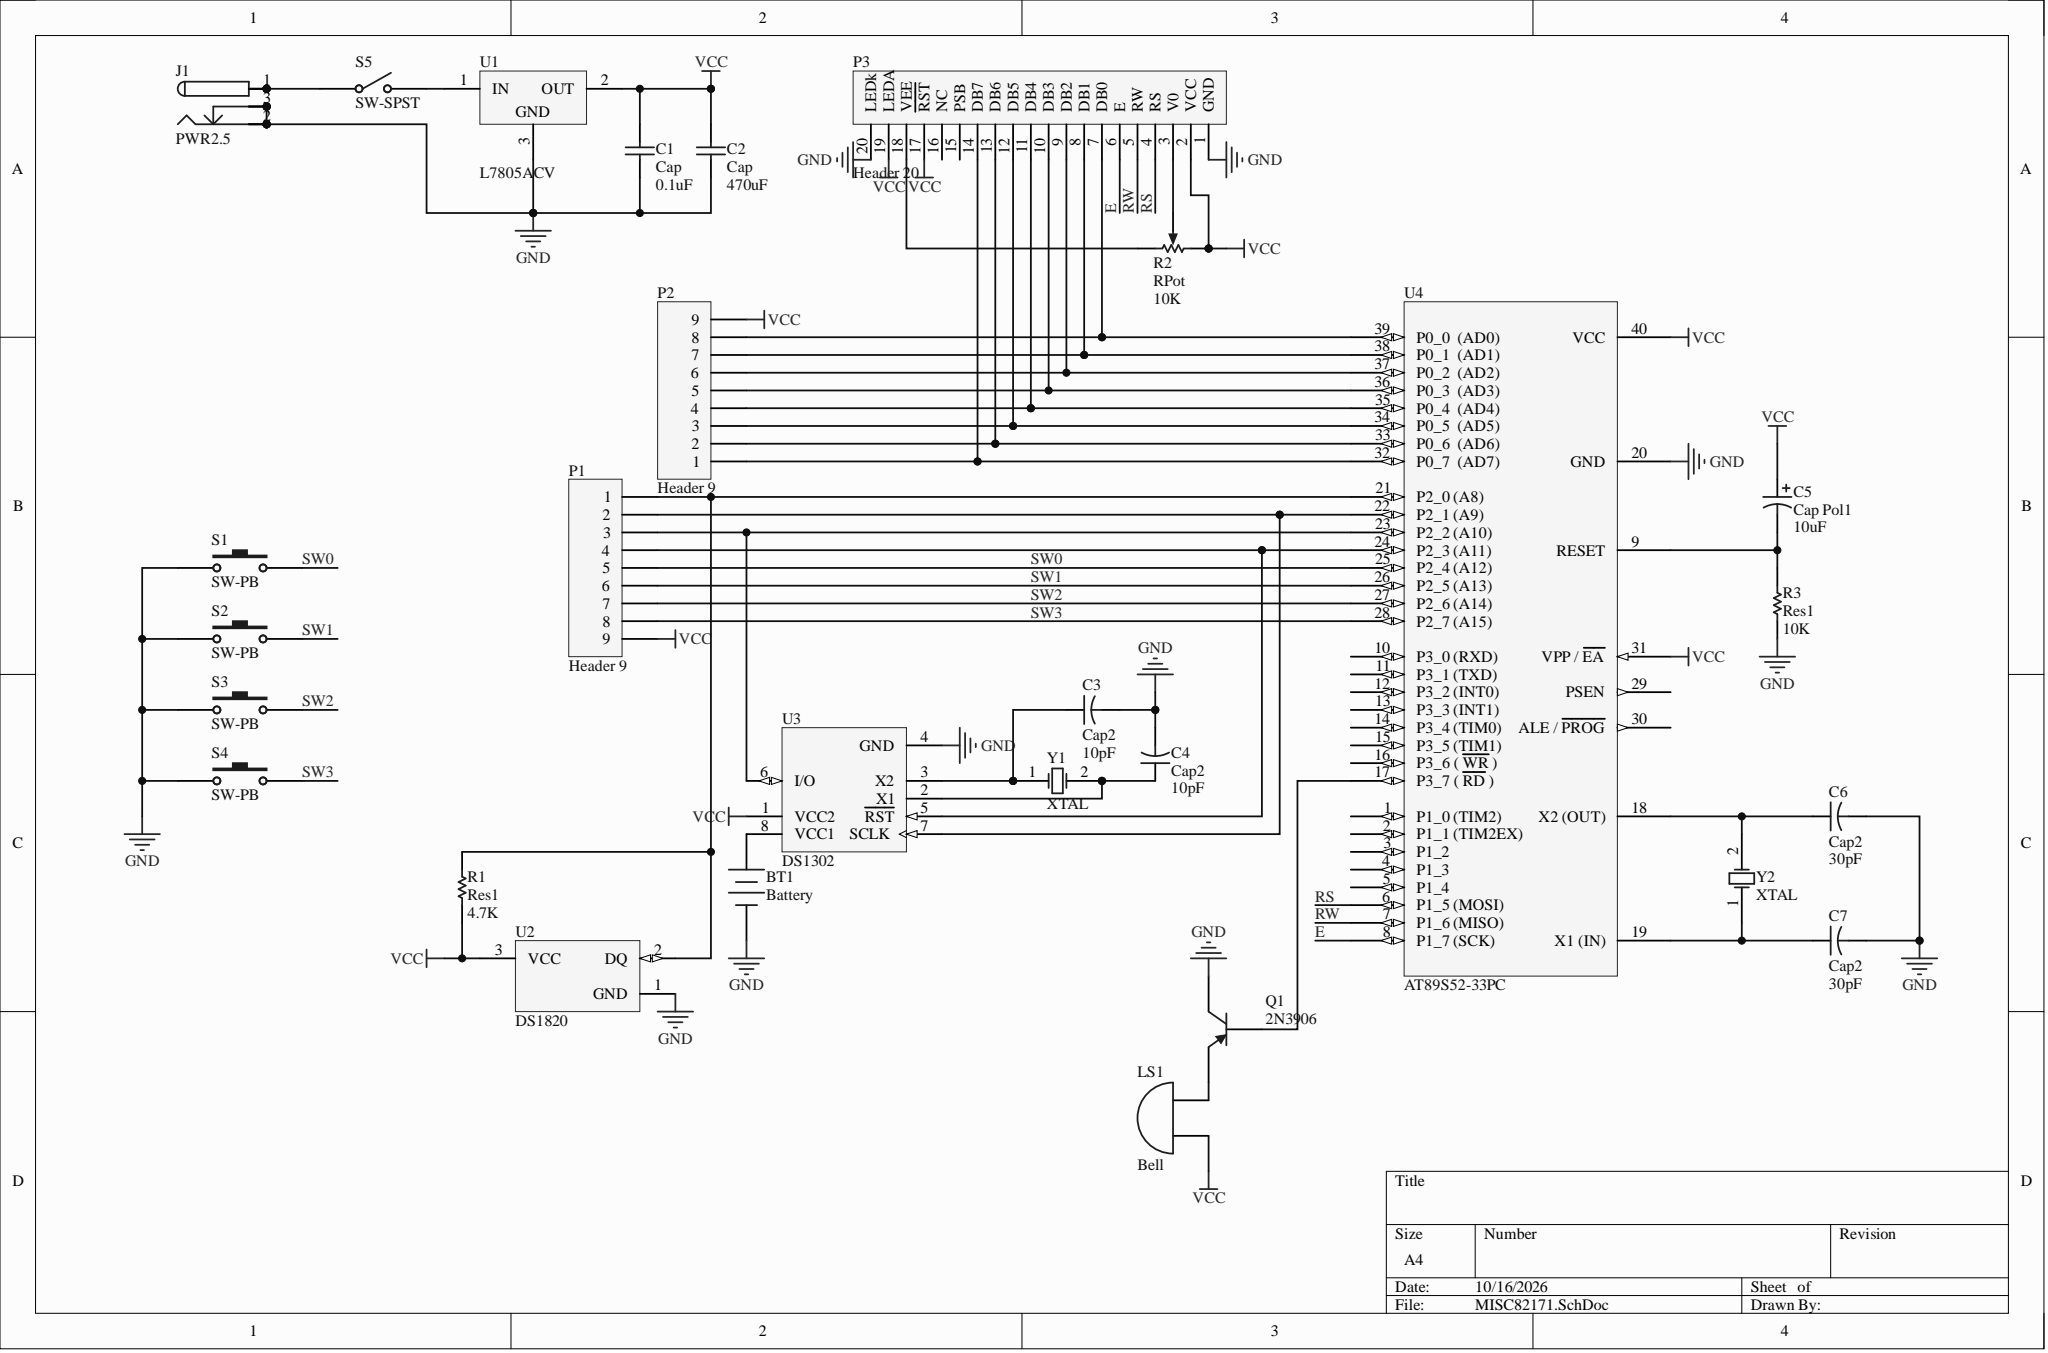Circuit board | Altium Designer | 28 parts | 33 nets
Bill of materials:
Comment,Description,Designator,Footprint,LibRef,Quantity
"Battery","Multicell Battery","BT1","3V电池","Battery","1"
"Cap","Capacitor","C1, C2","RAD-0.3","Cap","2"
"Cap2","Capacitor","C3, C4, C6, C7","CAPR5-4X5","Cap2","4"
"Cap Pol1","Polarized Capacitor (Radial)","C5","RB7.6-15","Cap Pol1","1"
"PWR2.5","Low Voltage Power Supply Connector","J1","DC","PWR2.5","1"
"Bell","Electrical Bell","LS1","BELL","Bell","1"
"Header 9","Header, 9-Pin","P1, P2","HDR1X9","Header 9","2"
"Header 20","Header, 20-Pin","P3","HDR1X20","Header 20","1"
"2N3906","PNP General Purpose Amplifier","Q1","TO-92A","2N3906","1"
"Res1","Resistor","R1, R3","AXIAL-0.3","Res1","2"
"RPot","Potentiometer","R2","VR4","RPot","1"
"SW-PB","Switch","S1, S2, S3, S4","SW4","SW-PB","4"
"SW-SPST","Single-Pole, Single-Throw Switch","S5","SPST-2","SW-SPST","1"
"L7805ACV","Precision 1A Regulator","U1","TO220ABN","L7805ACV","1"
"DS1820","1-Wire Digital Thermometer","U2","PR35","DS1820","1"
"DS1302","Trickle Charge Timekeeping Chip","U3","DIP8","DS1302","1"
"AT89S52-33PC","Atmel 8 Bit Micro 4.0-5.5V 33MHz 0-70 Deg C 40 PDIP (40P6) Package","U4","DIP40","AT89S52-33PC","1"
"XTAL","Crystal Oscillator","Y1","R38","XTAL","1"
"XTAL","Crystal Oscillator","Y2","XTAL2","XTAL","1"
Netlist (Protel format):
[
BT1
3V电池
Battery



]
[
C1
RAD-0.3
Cap



]
[
C2
RAD-0.3
Cap



]
[
C3
CAPR5-4X5
Cap2



]
[
C4
CAPR5-4X5
Cap2



]
[
C5
RB7.6-15
Cap Pol1



]
[
C6
CAPR5-4X5
Cap2



]
[
C7
CAPR5-4X5
Cap2



]
[
J1
DC
PWR2.5



]
[
LS1
BELL
Bell



]
[
P1
HDR1X9
Header 9



]
[
P2
HDR1X9
Header 9



]
[
P3
HDR1X20
Header 20



]
[
Q1
TO-92A
2N3906



]
[
R1
AXIAL-0.3
Res1



]
[
R2
VR4
RPot



]
[
R3
AXIAL-0.3
Res1



]
[
S1
SW4
SW-PB



]
[
S2
SW4
SW-PB



]
[
S3
SW4
SW-PB



]
[
S4
SW4
SW-PB



]
[
S5
SPST-2
SW-SPST



]
[
U1
TO220ABN
L7805ACV



]
[
U2
PR35
DS1820



]
[
U3
DIP8
DS1302



]
[
U4
DIP40
AT89S52-33PC



]
[
Y1
R38
XTAL



]
[
Y2
XTAL2
XTAL



]
(
VCC
C1-2
C2-2
C5-1
LS1-1
P1-9
P2-9
P3-2
P3-17
P3-19
R1-1
R2-1
U1-2
U2-3
U3-1
U4-31
U4-40
)
(
SW3
P1-8
S4-2
U4-28
)
(
SW2
P1-7
S3-2
U4-27
)
(
SW1
P1-6
S2-2
U4-26
)
(
SW0
P1-5
S1-2
U4-25
)
(
RW
P3-5
U4-7
)
(
RS
P3-4
U4-6
)
(
NetS5_2
S5-2
U1-1
)
(
NetQ1_2
Q1-2
U4-17
)
(
NetP3_18
P3-18
R2-2
)
(
NetP3_3
P3-3
R2-3
)
(
NetP2_8
P2-8
P3-7
U4-39
)
(
NetP2_7
P2-7
P3-8
U4-38
)
(
NetP2_6
P2-6
P3-9
U4-37
)
(
NetP2_5
P2-5
P3-10
U4-36
)
(
NetP2_4
P2-4
P3-11
U4-35
)
(
NetP2_3
P2-3
P3-12
U4-34
)
(
NetP2_2
P2-2
P3-13
U4-33
)
(
NetP2_1
P2-1
P3-14
U4-32
)
(
NetP1_4
P1-4
U3-5
U4-24
)
(
NetP1_3
P1-3
U3-6
U4-23
)
(
NetP1_2
P1-2
U3-7
U4-22
)
(
NetP1_1
P1-1
R1-2
U2-2
U4-21
)
(
NetLS1_2
LS1-2
Q1-1
)
(
NetJ1_1
J1-1
J1-1A
J1-1B
S5-1
)
(
NetC7_1
C7-1
U4-19
Y2-1
)
(
NetC6_1
C6-1
U4-18
Y2-2
)
(
NetC5_2
C5-2
R3-2
U4-9
)
(
NetC4_1
C4-1
U3-2
Y1-2
)
(
NetC3_1
C3-1
U3-3
Y1-1
)
(
NetBT1_1
BT1-1
U3-8
)
(
GND
BT1-2
C1-1
C2-1
C3-2
C4-2
C6-2
C7-2
J1-2
J1-2A
J1-2B
J1-3
J1-3A
J1-3B
P3-1
P3-20
Q1-3
R3-1
S1-1
S2-1
S3-1
S4-1
U1-3
U2-1
U3-4
U4-20
)
(
E
P3-6
U4-8
)